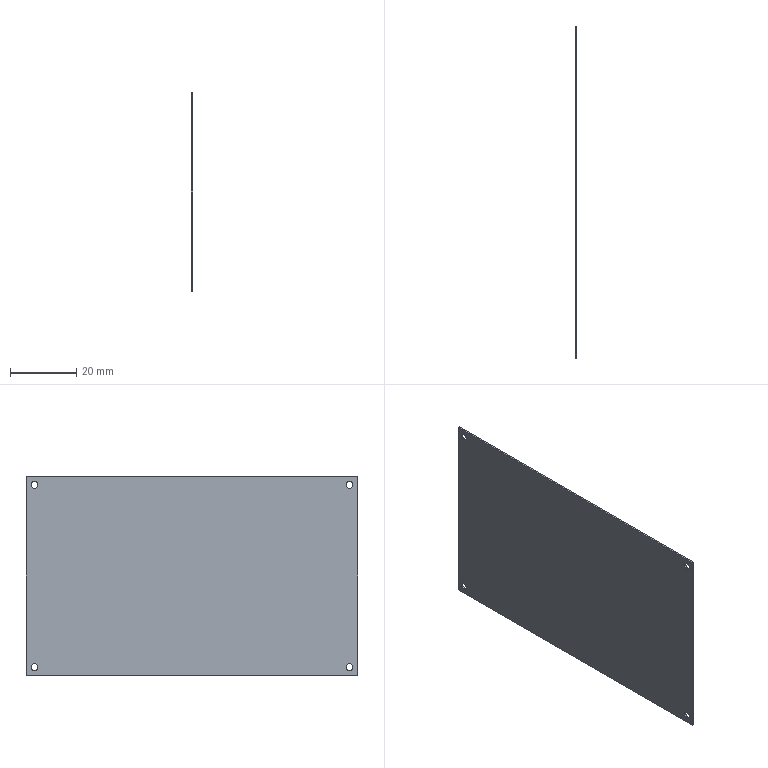Part | STEP file | 车灯-后视镜_id86_x_t | 1 solid | 10 faces | box 0.5 x 100 x 60 mm | volume 2994 mm3 | plane 6 | cylinder 4 | commonest cylinder face diameters 2 x4
STEP:
#1=CARTESIAN_POINT('',(-250.,197.5,-239.));
#2=VERTEX_POINT('',#1);
#3=CARTESIAN_POINT('',(-250.,197.5,-238.));
#4=DIRECTION('',(-1.,0.,0.));
#5=DIRECTION('',(0.,0.,-1.));
#6=AXIS2_PLACEMENT_3D('',#3,#4,#5);
#7=CIRCLE('',#6,1.);
#8=EDGE_CURVE('',#2,#2,#7,.T.);
#9=ORIENTED_EDGE('',*,*,#8,.T.);
#10=EDGE_LOOP('',(#9));
#11=FACE_BOUND('',#10,.T.);
#12=CARTESIAN_POINT('',(-250.,197.5,-294.));
#13=VERTEX_POINT('',#12);
#14=CARTESIAN_POINT('',(-250.,197.5,-293.));
#15=DIRECTION('',(-1.,0.,0.));
#16=DIRECTION('',(0.,0.,-1.));
#17=AXIS2_PLACEMENT_3D('',#14,#15,#16);
#18=CIRCLE('',#17,1.);
#19=EDGE_CURVE('',#13,#13,#18,.T.);
#20=ORIENTED_EDGE('',*,*,#19,.T.);
#21=EDGE_LOOP('',(#20));
#22=FACE_BOUND('',#21,.T.);
#23=CARTESIAN_POINT('',(-250.,102.5,-294.));
#24=VERTEX_POINT('',#23);
#25=CARTESIAN_POINT('',(-250.,102.5,-293.));
#26=DIRECTION('',(-1.,0.,0.));
#27=DIRECTION('',(0.,0.,-1.));
#28=AXIS2_PLACEMENT_3D('',#25,#26,#27);
#29=CIRCLE('',#28,1.);
#30=EDGE_CURVE('',#24,#24,#29,.T.);
#31=ORIENTED_EDGE('',*,*,#30,.T.);
#32=EDGE_LOOP('',(#31));
#33=FACE_BOUND('',#32,.T.);
#34=CARTESIAN_POINT('',(-250.,102.5,-239.));
#35=VERTEX_POINT('',#34);
#36=CARTESIAN_POINT('',(-250.,102.5,-238.));
#37=DIRECTION('',(-1.,0.,0.));
#38=DIRECTION('',(0.,0.,-1.));
#39=AXIS2_PLACEMENT_3D('',#36,#37,#38);
#40=CIRCLE('',#39,1.);
#41=EDGE_CURVE('',#35,#35,#40,.T.);
#42=ORIENTED_EDGE('',*,*,#41,.T.);
#43=EDGE_LOOP('',(#42));
#44=FACE_BOUND('',#43,.T.);
#45=CARTESIAN_POINT('',(-250.,200.,-295.5));
#46=VERTEX_POINT('',#45);
#47=CARTESIAN_POINT('',(-250.,200.,-235.5));
#48=VERTEX_POINT('',#47);
#49=CARTESIAN_POINT('',(-250.,200.,-295.5));
#50=DIRECTION('',(0.,0.,1.));
#51=VECTOR('',#50,1.);
#52=LINE('',#49,#51);
#53=EDGE_CURVE('',#46,#48,#52,.T.);
#54=ORIENTED_EDGE('',*,*,#53,.T.);
#55=CARTESIAN_POINT('',(-250.,100.,-235.5));
#56=VERTEX_POINT('',#55);
#57=CARTESIAN_POINT('',(-250.,425.,-235.5));
#58=DIRECTION('',(0.,-1.,0.));
#59=VECTOR('',#58,1.);
#60=LINE('',#57,#59);
#61=EDGE_CURVE('',#48,#56,#60,.T.);
#62=ORIENTED_EDGE('',*,*,#61,.T.);
#63=CARTESIAN_POINT('',(-250.,100.,-295.5));
#64=VERTEX_POINT('',#63);
#65=CARTESIAN_POINT('',(-250.,100.,-295.5));
#66=DIRECTION('',(0.,0.,1.));
#67=VECTOR('',#66,1.);
#68=LINE('',#65,#67);
#69=EDGE_CURVE('',#64,#56,#68,.T.);
#70=ORIENTED_EDGE('',*,*,#69,.F.);
#71=CARTESIAN_POINT('',(-250.,425.,-295.5));
#72=DIRECTION('',(0.,-1.,0.));
#73=VECTOR('',#72,1.);
#74=LINE('',#71,#73);
#75=EDGE_CURVE('',#46,#64,#74,.T.);
#76=ORIENTED_EDGE('',*,*,#75,.F.);
#77=EDGE_LOOP('',(#54,#62,#70,#76));
#78=FACE_BOUND('',#77,.T.);
#79=CARTESIAN_POINT('',(-250.,425.,-295.5));
#80=DIRECTION('',(1.,0.,0.));
#81=DIRECTION('',(0.,-1.,0.));
#82=AXIS2_PLACEMENT_3D('',#79,#80,#81);
#83=PLANE('',#82);
#84=ADVANCED_FACE('',(#11,#22,#33,#44,#78),#83,.T.);
#85=ORIENTED_EDGE('',*,*,#69,.T.);
#86=CARTESIAN_POINT('',(-250.5,100.,-235.5));
#87=VERTEX_POINT('',#86);
#88=CARTESIAN_POINT('',(-250.,100.,-235.5));
#89=DIRECTION('',(-1.,0.,0.));
#90=VECTOR('',#89,1.);
#91=LINE('',#88,#90);
#92=EDGE_CURVE('',#56,#87,#91,.T.);
#93=ORIENTED_EDGE('',*,*,#92,.T.);
#94=CARTESIAN_POINT('',(-250.5,100.,-295.5));
#95=VERTEX_POINT('',#94);
#96=CARTESIAN_POINT('',(-250.5,100.,-295.5));
#97=DIRECTION('',(0.,0.,1.));
#98=VECTOR('',#97,1.);
#99=LINE('',#96,#98);
#100=EDGE_CURVE('',#95,#87,#99,.T.);
#101=ORIENTED_EDGE('',*,*,#100,.F.);
#102=CARTESIAN_POINT('',(-250.,100.,-295.5));
#103=DIRECTION('',(-1.,0.,0.));
#104=VECTOR('',#103,1.);
#105=LINE('',#102,#104);
#106=EDGE_CURVE('',#64,#95,#105,.T.);
#107=ORIENTED_EDGE('',*,*,#106,.F.);
#108=EDGE_LOOP('',(#85,#93,#101,#107));
#109=FACE_OUTER_BOUND('',#108,.T.);
#110=CARTESIAN_POINT('',(-250.,100.,-295.5));
#111=DIRECTION('',(0.,-1.,0.));
#112=DIRECTION('',(-1.,0.,0.));
#113=AXIS2_PLACEMENT_3D('',#110,#111,#112);
#114=PLANE('',#113);
#115=ADVANCED_FACE('',(#109),#114,.T.);
#116=CARTESIAN_POINT('',(-250.5,197.5,-239.));
#117=VERTEX_POINT('',#116);
#118=CARTESIAN_POINT('',(-250.5,197.5,-238.));
#119=DIRECTION('',(1.,0.,0.));
#120=DIRECTION('',(0.,0.,-1.));
#121=AXIS2_PLACEMENT_3D('',#118,#119,#120);
#122=CIRCLE('',#121,1.);
#123=EDGE_CURVE('',#117,#117,#122,.T.);
#124=ORIENTED_EDGE('',*,*,#123,.T.);
#125=EDGE_LOOP('',(#124));
#126=FACE_BOUND('',#125,.T.);
#127=CARTESIAN_POINT('',(-250.5,197.5,-294.));
#128=VERTEX_POINT('',#127);
#129=CARTESIAN_POINT('',(-250.5,197.5,-293.));
#130=DIRECTION('',(1.,0.,0.));
#131=DIRECTION('',(0.,0.,-1.));
#132=AXIS2_PLACEMENT_3D('',#129,#130,#131);
#133=CIRCLE('',#132,1.);
#134=EDGE_CURVE('',#128,#128,#133,.T.);
#135=ORIENTED_EDGE('',*,*,#134,.T.);
#136=EDGE_LOOP('',(#135));
#137=FACE_BOUND('',#136,.T.);
#138=CARTESIAN_POINT('',(-250.5,102.5,-294.));
#139=VERTEX_POINT('',#138);
#140=CARTESIAN_POINT('',(-250.5,102.5,-293.));
#141=DIRECTION('',(1.,0.,0.));
#142=DIRECTION('',(0.,0.,-1.));
#143=AXIS2_PLACEMENT_3D('',#140,#141,#142);
#144=CIRCLE('',#143,1.);
#145=EDGE_CURVE('',#139,#139,#144,.T.);
#146=ORIENTED_EDGE('',*,*,#145,.T.);
#147=EDGE_LOOP('',(#146));
#148=FACE_BOUND('',#147,.T.);
#149=CARTESIAN_POINT('',(-250.5,102.5,-239.));
#150=VERTEX_POINT('',#149);
#151=CARTESIAN_POINT('',(-250.5,102.5,-238.));
#152=DIRECTION('',(1.,0.,0.));
#153=DIRECTION('',(0.,0.,-1.));
#154=AXIS2_PLACEMENT_3D('',#151,#152,#153);
#155=CIRCLE('',#154,1.);
#156=EDGE_CURVE('',#150,#150,#155,.T.);
#157=ORIENTED_EDGE('',*,*,#156,.T.);
#158=EDGE_LOOP('',(#157));
#159=FACE_BOUND('',#158,.T.);
#160=ORIENTED_EDGE('',*,*,#100,.T.);
#161=CARTESIAN_POINT('',(-250.5,200.,-235.5));
#162=VERTEX_POINT('',#161);
#163=CARTESIAN_POINT('',(-250.5,425.,-235.5));
#164=DIRECTION('',(0.,-1.,0.));
#165=VECTOR('',#164,1.);
#166=LINE('',#163,#165);
#167=EDGE_CURVE('',#162,#87,#166,.T.);
#168=ORIENTED_EDGE('',*,*,#167,.F.);
#169=CARTESIAN_POINT('',(-250.5,200.,-295.5));
#170=VERTEX_POINT('',#169);
#171=CARTESIAN_POINT('',(-250.5,200.,-295.5));
#172=DIRECTION('',(0.,0.,1.));
#173=VECTOR('',#172,1.);
#174=LINE('',#171,#173);
#175=EDGE_CURVE('',#170,#162,#174,.T.);
#176=ORIENTED_EDGE('',*,*,#175,.F.);
#177=CARTESIAN_POINT('',(-250.5,425.,-295.5));
#178=DIRECTION('',(0.,-1.,0.));
#179=VECTOR('',#178,1.);
#180=LINE('',#177,#179);
#181=EDGE_CURVE('',#170,#95,#180,.T.);
#182=ORIENTED_EDGE('',*,*,#181,.T.);
#183=EDGE_LOOP('',(#160,#168,#176,#182));
#184=FACE_BOUND('',#183,.T.);
#185=CARTESIAN_POINT('',(-250.5,425.,-295.5));
#186=DIRECTION('',(1.,0.,0.));
#187=DIRECTION('',(0.,-1.,0.));
#188=AXIS2_PLACEMENT_3D('',#185,#186,#187);
#189=PLANE('',#188);
#190=ADVANCED_FACE('',(#126,#137,#148,#159,#184),#189,.F.);
#191=CARTESIAN_POINT('',(-250.,200.,-295.5));
#192=DIRECTION('',(-1.,0.,0.));
#193=VECTOR('',#192,1.);
#194=LINE('',#191,#193);
#195=EDGE_CURVE('',#46,#170,#194,.T.);
#196=ORIENTED_EDGE('',*,*,#195,.T.);
#197=ORIENTED_EDGE('',*,*,#175,.T.);
#198=CARTESIAN_POINT('',(-250.,200.,-235.5));
#199=DIRECTION('',(-1.,0.,0.));
#200=VECTOR('',#199,1.);
#201=LINE('',#198,#200);
#202=EDGE_CURVE('',#48,#162,#201,.T.);
#203=ORIENTED_EDGE('',*,*,#202,.F.);
#204=ORIENTED_EDGE('',*,*,#53,.F.);
#205=EDGE_LOOP('',(#196,#197,#203,#204));
#206=FACE_OUTER_BOUND('',#205,.T.);
#207=CARTESIAN_POINT('',(-250.,200.,-295.5));
#208=DIRECTION('',(0.,-1.,0.));
#209=DIRECTION('',(-1.,0.,0.));
#210=AXIS2_PLACEMENT_3D('',#207,#208,#209);
#211=PLANE('',#210);
#212=ADVANCED_FACE('',(#206),#211,.F.);
#213=ORIENTED_EDGE('',*,*,#167,.T.);
#214=ORIENTED_EDGE('',*,*,#92,.F.);
#215=ORIENTED_EDGE('',*,*,#61,.F.);
#216=ORIENTED_EDGE('',*,*,#202,.T.);
#217=EDGE_LOOP('',(#213,#214,#215,#216));
#218=FACE_OUTER_BOUND('',#217,.T.);
#219=CARTESIAN_POINT('',(-250.,425.,-235.5));
#220=DIRECTION('',(0.,0.,-1.));
#221=DIRECTION('',(-1.,0.,0.));
#222=AXIS2_PLACEMENT_3D('',#219,#220,#221);
#223=PLANE('',#222);
#224=ADVANCED_FACE('',(#218),#223,.F.);
#225=ORIENTED_EDGE('',*,*,#181,.F.);
#226=ORIENTED_EDGE('',*,*,#195,.F.);
#227=ORIENTED_EDGE('',*,*,#75,.T.);
#228=ORIENTED_EDGE('',*,*,#106,.T.);
#229=EDGE_LOOP('',(#225,#226,#227,#228));
#230=FACE_OUTER_BOUND('',#229,.T.);
#231=CARTESIAN_POINT('',(-250.,425.,-295.5));
#232=DIRECTION('',(0.,0.,-1.));
#233=DIRECTION('',(-1.,0.,0.));
#234=AXIS2_PLACEMENT_3D('',#231,#232,#233);
#235=PLANE('',#234);
#236=ADVANCED_FACE('',(#230),#235,.T.);
#237=ORIENTED_EDGE('',*,*,#156,.F.);
#238=EDGE_LOOP('',(#237));
#239=FACE_BOUND('',#238,.T.);
#240=ORIENTED_EDGE('',*,*,#41,.F.);
#241=EDGE_LOOP('',(#240));
#242=FACE_BOUND('',#241,.T.);
#243=CARTESIAN_POINT('',(-250.5,102.5,-238.));
#244=DIRECTION('',(1.,0.,0.));
#245=DIRECTION('',(0.,0.,-1.));
#246=AXIS2_PLACEMENT_3D('',#243,#244,#245);
#247=CYLINDRICAL_SURFACE('',#246,1.);
#248=ADVANCED_FACE('',(#239,#242),#247,.F.);
#249=ORIENTED_EDGE('',*,*,#145,.F.);
#250=EDGE_LOOP('',(#249));
#251=FACE_BOUND('',#250,.T.);
#252=ORIENTED_EDGE('',*,*,#30,.F.);
#253=EDGE_LOOP('',(#252));
#254=FACE_BOUND('',#253,.T.);
#255=CARTESIAN_POINT('',(-250.5,102.5,-293.));
#256=DIRECTION('',(1.,0.,0.));
#257=DIRECTION('',(0.,0.,-1.));
#258=AXIS2_PLACEMENT_3D('',#255,#256,#257);
#259=CYLINDRICAL_SURFACE('',#258,1.);
#260=ADVANCED_FACE('',(#251,#254),#259,.F.);
#261=ORIENTED_EDGE('',*,*,#134,.F.);
#262=EDGE_LOOP('',(#261));
#263=FACE_BOUND('',#262,.T.);
#264=ORIENTED_EDGE('',*,*,#19,.F.);
#265=EDGE_LOOP('',(#264));
#266=FACE_BOUND('',#265,.T.);
#267=CARTESIAN_POINT('',(-250.5,197.5,-293.));
#268=DIRECTION('',(1.,0.,0.));
#269=DIRECTION('',(0.,0.,-1.));
#270=AXIS2_PLACEMENT_3D('',#267,#268,#269);
#271=CYLINDRICAL_SURFACE('',#270,1.);
#272=ADVANCED_FACE('',(#263,#266),#271,.F.);
#273=ORIENTED_EDGE('',*,*,#123,.F.);
#274=EDGE_LOOP('',(#273));
#275=FACE_BOUND('',#274,.T.);
#276=ORIENTED_EDGE('',*,*,#8,.F.);
#277=EDGE_LOOP('',(#276));
#278=FACE_BOUND('',#277,.T.);
#279=CARTESIAN_POINT('',(-250.5,197.5,-238.));
#280=DIRECTION('',(1.,0.,0.));
#281=DIRECTION('',(0.,0.,-1.));
#282=AXIS2_PLACEMENT_3D('',#279,#280,#281);
#283=CYLINDRICAL_SURFACE('',#282,1.);
#284=ADVANCED_FACE('',(#275,#278),#283,.F.);
#285=CLOSED_SHELL('',(#84,#115,#190,#212,#224,#236,#248,#260,#272,#284));
#286=MANIFOLD_SOLID_BREP('',#285);
#287=(LENGTH_UNIT()NAMED_UNIT(*)SI_UNIT(.MILLI.,.METRE.));
#288=UNCERTAINTY_MEASURE_WITH_UNIT(LENGTH_MEASURE(0.00002),#287,'','');
#289=(NAMED_UNIT(*)PLANE_ANGLE_UNIT()SI_UNIT($,.RADIAN.));
#290=PLANE_ANGLE_MEASURE_WITH_UNIT(PLANE_ANGLE_MEASURE(0.01745),#289);
#291=DIMENSIONAL_EXPONENTS(0.,0.,0.,0.,0.,0.,0.);
#292=(CONVERSION_BASED_UNIT('DEGREE',#290)NAMED_UNIT(#291)PLANE_ANGLE_UNIT());
#293=(NAMED_UNIT(*)SI_UNIT($,.STERADIAN.)SOLID_ANGLE_UNIT());
#294=(GEOMETRIC_REPRESENTATION_CONTEXT(3)GLOBAL_UNCERTAINTY_ASSIGNED_CONTEXT((#288))GLOBAL_UNIT_ASSIGNED_CONTEXT((#287,#292,#293))REPRESENTATION_CONTEXT('',''));
#295=ADVANCED_BREP_SHAPE_REPRESENTATION('',(#286),#294);